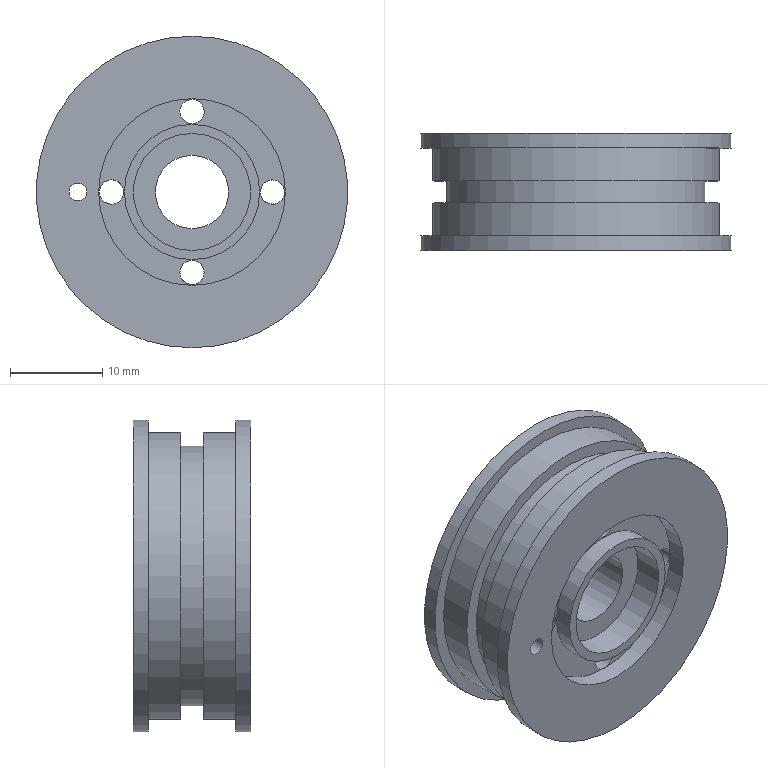Part | NX | features piston 2 | 1 solid | 23 faces | box 33.782 x 12.7 x 33.782 mm | volume 8306 mm3 | cylinder 14 | plane 9 | commonest cylinder face diameters 2.642 x4 31.115 x2 33.782 x2 1.93 x1 7.95 x1 12.7 x1
STEP:
#1=CARTESIAN_POINT('',(0.,0.,-7.333));
#2=VERTEX_POINT('',#1);
#3=CARTESIAN_POINT('',(0.,0.,0.));
#4=DIRECTION('',(0.,-1.,0.));
#5=DIRECTION('',(0.,0.,-1.));
#6=AXIS2_PLACEMENT_3D('',#3,#4,#5);
#7=CIRCLE('',#6,7.333);
#8=EDGE_CURVE('',#2,#2,#7,.F.);
#9=ORIENTED_EDGE('',*,*,#8,.F.);
#10=EDGE_LOOP('',(#9));
#11=FACE_BOUND('',#10,.T.);
#12=CARTESIAN_POINT('',(0.,0.,-6.35));
#13=VERTEX_POINT('',#12);
#14=CARTESIAN_POINT('',(0.,0.,0.));
#15=DIRECTION('',(0.,-1.,0.));
#16=DIRECTION('',(0.,0.,-1.));
#17=AXIS2_PLACEMENT_3D('',#14,#15,#16);
#18=CIRCLE('',#17,6.35);
#19=EDGE_CURVE('',#13,#13,#18,.T.);
#20=ORIENTED_EDGE('',*,*,#19,.F.);
#21=EDGE_LOOP('',(#20));
#22=FACE_BOUND('',#21,.T.);
#23=CARTESIAN_POINT('',(6.35,0.,0.));
#24=DIRECTION('',(0.,-1.,0.));
#25=DIRECTION('',(0.,0.,-1.));
#26=AXIS2_PLACEMENT_3D('',#23,#24,#25);
#27=PLANE('',#26);
#28=ADVANCED_FACE('',(#11,#22),#27,.T.);
#29=CARTESIAN_POINT('',(8.73,12.7,1.321));
#30=VERTEX_POINT('',#29);
#31=CARTESIAN_POINT('',(8.73,12.7,0.));
#32=DIRECTION('',(0.,1.,0.));
#33=DIRECTION('',(0.,0.,1.));
#34=AXIS2_PLACEMENT_3D('',#31,#32,#33);
#35=CIRCLE('',#34,1.321);
#36=EDGE_CURVE('',#30,#30,#35,.F.);
#37=ORIENTED_EDGE('',*,*,#36,.T.);
#38=EDGE_LOOP('',(#37));
#39=FACE_BOUND('',#38,.T.);
#40=CARTESIAN_POINT('',(-8.73,12.7,1.321));
#41=VERTEX_POINT('',#40);
#42=CARTESIAN_POINT('',(-8.73,12.7,0.));
#43=DIRECTION('',(0.,1.,0.));
#44=DIRECTION('',(0.,0.,1.));
#45=AXIS2_PLACEMENT_3D('',#42,#43,#44);
#46=CIRCLE('',#45,1.321);
#47=EDGE_CURVE('',#41,#41,#46,.F.);
#48=ORIENTED_EDGE('',*,*,#47,.T.);
#49=EDGE_LOOP('',(#48));
#50=FACE_BOUND('',#49,.T.);
#51=CARTESIAN_POINT('',(0.,12.7,-16.891));
#52=VERTEX_POINT('',#51);
#53=CARTESIAN_POINT('',(0.,12.7,0.));
#54=DIRECTION('',(0.,-1.,0.));
#55=DIRECTION('',(0.,0.,-1.));
#56=AXIS2_PLACEMENT_3D('',#53,#54,#55);
#57=CIRCLE('',#56,16.891);
#58=EDGE_CURVE('',#52,#52,#57,.T.);
#59=ORIENTED_EDGE('',*,*,#58,.F.);
#60=EDGE_LOOP('',(#59));
#61=FACE_BOUND('',#60,.T.);
#62=CARTESIAN_POINT('',(0.,12.7,-3.975));
#63=VERTEX_POINT('',#62);
#64=CARTESIAN_POINT('',(0.,12.7,0.));
#65=DIRECTION('',(0.,-1.,0.));
#66=DIRECTION('',(0.,0.,-1.));
#67=AXIS2_PLACEMENT_3D('',#64,#65,#66);
#68=CIRCLE('',#67,3.975);
#69=EDGE_CURVE('',#63,#63,#68,.T.);
#70=ORIENTED_EDGE('',*,*,#69,.T.);
#71=EDGE_LOOP('',(#70));
#72=FACE_BOUND('',#71,.T.);
#73=CARTESIAN_POINT('',(-12.383,12.7,0.9652));
#74=VERTEX_POINT('',#73);
#75=CARTESIAN_POINT('',(-12.383,12.7,0.));
#76=DIRECTION('',(0.,1.,0.));
#77=DIRECTION('',(0.,0.,1.));
#78=AXIS2_PLACEMENT_3D('',#75,#76,#77);
#79=CIRCLE('',#78,0.9652);
#80=EDGE_CURVE('',#74,#74,#79,.F.);
#81=ORIENTED_EDGE('',*,*,#80,.T.);
#82=EDGE_LOOP('',(#81));
#83=FACE_BOUND('',#82,.T.);
#84=CARTESIAN_POINT('',(0.,12.7,-7.409));
#85=VERTEX_POINT('',#84);
#86=CARTESIAN_POINT('',(0.,12.7,-8.73));
#87=DIRECTION('',(0.,1.,0.));
#88=DIRECTION('',(0.,0.,1.));
#89=AXIS2_PLACEMENT_3D('',#86,#87,#88);
#90=CIRCLE('',#89,1.321);
#91=EDGE_CURVE('',#85,#85,#90,.F.);
#92=ORIENTED_EDGE('',*,*,#91,.T.);
#93=EDGE_LOOP('',(#92));
#94=FACE_BOUND('',#93,.T.);
#95=CARTESIAN_POINT('',(0.,12.7,10.051));
#96=VERTEX_POINT('',#95);
#97=CARTESIAN_POINT('',(0.,12.7,8.73));
#98=DIRECTION('',(0.,1.,0.));
#99=DIRECTION('',(0.,0.,1.));
#100=AXIS2_PLACEMENT_3D('',#97,#98,#99);
#101=CIRCLE('',#100,1.321);
#102=EDGE_CURVE('',#96,#96,#101,.F.);
#103=ORIENTED_EDGE('',*,*,#102,.T.);
#104=EDGE_LOOP('',(#103));
#105=FACE_BOUND('',#104,.T.);
#106=CARTESIAN_POINT('',(16.891,12.7,0.));
#107=DIRECTION('',(0.,1.,0.));
#108=DIRECTION('',(0.,0.,1.));
#109=AXIS2_PLACEMENT_3D('',#106,#107,#108);
#110=PLANE('',#109);
#111=ADVANCED_FACE('',(#39,#50,#61,#72,#83,#94,#105),#110,.T.);
#112=CARTESIAN_POINT('',(0.,0.,-10.127));
#113=VERTEX_POINT('',#112);
#114=CARTESIAN_POINT('',(0.,0.,0.));
#115=DIRECTION('',(0.,-1.,0.));
#116=DIRECTION('',(0.,0.,-1.));
#117=AXIS2_PLACEMENT_3D('',#114,#115,#116);
#118=CIRCLE('',#117,10.127);
#119=EDGE_CURVE('',#113,#113,#118,.T.);
#120=ORIENTED_EDGE('',*,*,#119,.F.);
#121=EDGE_LOOP('',(#120));
#122=FACE_BOUND('',#121,.T.);
#123=CARTESIAN_POINT('',(0.,0.,-16.891));
#124=VERTEX_POINT('',#123);
#125=CARTESIAN_POINT('',(0.,0.,0.));
#126=DIRECTION('',(0.,-1.,0.));
#127=DIRECTION('',(0.,0.,-1.));
#128=AXIS2_PLACEMENT_3D('',#125,#126,#127);
#129=CIRCLE('',#128,16.891);
#130=EDGE_CURVE('',#124,#124,#129,.T.);
#131=ORIENTED_EDGE('',*,*,#130,.T.);
#132=EDGE_LOOP('',(#131));
#133=FACE_BOUND('',#132,.T.);
#134=CARTESIAN_POINT('',(-12.383,0.,-0.9652));
#135=VERTEX_POINT('',#134);
#136=CARTESIAN_POINT('',(-12.383,0.,0.));
#137=DIRECTION('',(0.,-1.,0.));
#138=DIRECTION('',(0.,0.,-1.));
#139=AXIS2_PLACEMENT_3D('',#136,#137,#138);
#140=CIRCLE('',#139,0.9652);
#141=EDGE_CURVE('',#135,#135,#140,.F.);
#142=ORIENTED_EDGE('',*,*,#141,.T.);
#143=EDGE_LOOP('',(#142));
#144=FACE_BOUND('',#143,.T.);
#145=CARTESIAN_POINT('',(6.35,0.,0.));
#146=DIRECTION('',(0.,-1.,0.));
#147=DIRECTION('',(0.,0.,-1.));
#148=AXIS2_PLACEMENT_3D('',#145,#146,#147);
#149=PLANE('',#148);
#150=ADVANCED_FACE('',(#122,#133,#144),#149,.T.);
#151=CARTESIAN_POINT('',(0.,3.175,-3.975));
#152=VERTEX_POINT('',#151);
#153=CARTESIAN_POINT('',(0.,3.175,0.));
#154=DIRECTION('',(0.,-1.,0.));
#155=DIRECTION('',(0.,0.,-1.));
#156=AXIS2_PLACEMENT_3D('',#153,#154,#155);
#157=CIRCLE('',#156,3.975);
#158=EDGE_CURVE('',#152,#152,#157,.T.);
#159=ORIENTED_EDGE('',*,*,#158,.T.);
#160=EDGE_LOOP('',(#159));
#161=FACE_BOUND('',#160,.T.);
#162=ORIENTED_EDGE('',*,*,#69,.F.);
#163=EDGE_LOOP('',(#162));
#164=FACE_BOUND('',#163,.T.);
#165=CARTESIAN_POINT('',(0.,0.,0.));
#166=DIRECTION('',(0.,-1.,0.));
#167=DIRECTION('',(0.,0.,-1.));
#168=AXIS2_PLACEMENT_3D('',#165,#166,#167);
#169=CYLINDRICAL_SURFACE('',#168,3.975);
#170=ADVANCED_FACE('',(#161,#164),#169,.F.);
#171=CARTESIAN_POINT('',(0.,3.175,-6.35));
#172=VERTEX_POINT('',#171);
#173=CARTESIAN_POINT('',(0.,3.175,0.));
#174=DIRECTION('',(0.,-1.,0.));
#175=DIRECTION('',(0.,0.,-1.));
#176=AXIS2_PLACEMENT_3D('',#173,#174,#175);
#177=CIRCLE('',#176,6.35);
#178=EDGE_CURVE('',#172,#172,#177,.T.);
#179=ORIENTED_EDGE('',*,*,#178,.T.);
#180=EDGE_LOOP('',(#179));
#181=FACE_BOUND('',#180,.T.);
#182=ORIENTED_EDGE('',*,*,#158,.F.);
#183=EDGE_LOOP('',(#182));
#184=FACE_BOUND('',#183,.T.);
#185=CARTESIAN_POINT('',(3.975,3.175,0.));
#186=DIRECTION('',(0.,-1.,0.));
#187=DIRECTION('',(0.,0.,-1.));
#188=AXIS2_PLACEMENT_3D('',#185,#186,#187);
#189=PLANE('',#188);
#190=ADVANCED_FACE('',(#181,#184),#189,.T.);
#191=ORIENTED_EDGE('',*,*,#19,.T.);
#192=EDGE_LOOP('',(#191));
#193=FACE_BOUND('',#192,.T.);
#194=ORIENTED_EDGE('',*,*,#178,.F.);
#195=EDGE_LOOP('',(#194));
#196=FACE_BOUND('',#195,.T.);
#197=CARTESIAN_POINT('',(0.,0.,0.));
#198=DIRECTION('',(0.,-1.,0.));
#199=DIRECTION('',(0.,0.,-1.));
#200=AXIS2_PLACEMENT_3D('',#197,#198,#199);
#201=CYLINDRICAL_SURFACE('',#200,6.35);
#202=ADVANCED_FACE('',(#193,#196),#201,.F.);
#203=CARTESIAN_POINT('',(0.,1.587,-16.891));
#204=VERTEX_POINT('',#203);
#205=CARTESIAN_POINT('',(0.,1.587,0.));
#206=DIRECTION('',(0.,-1.,0.));
#207=DIRECTION('',(0.,0.,-1.));
#208=AXIS2_PLACEMENT_3D('',#205,#206,#207);
#209=CIRCLE('',#208,16.891);
#210=EDGE_CURVE('',#204,#204,#209,.T.);
#211=ORIENTED_EDGE('',*,*,#210,.T.);
#212=EDGE_LOOP('',(#211));
#213=FACE_BOUND('',#212,.T.);
#214=ORIENTED_EDGE('',*,*,#130,.F.);
#215=EDGE_LOOP('',(#214));
#216=FACE_BOUND('',#215,.T.);
#217=CARTESIAN_POINT('',(0.,0.,0.));
#218=DIRECTION('',(0.,-1.,0.));
#219=DIRECTION('',(0.,0.,-1.));
#220=AXIS2_PLACEMENT_3D('',#217,#218,#219);
#221=CYLINDRICAL_SURFACE('',#220,16.891);
#222=ADVANCED_FACE('',(#213,#216),#221,.T.);
#223=CARTESIAN_POINT('',(0.,1.587,-15.557));
#224=VERTEX_POINT('',#223);
#225=CARTESIAN_POINT('',(0.,1.587,0.));
#226=DIRECTION('',(0.,-1.,0.));
#227=DIRECTION('',(0.,0.,-1.));
#228=AXIS2_PLACEMENT_3D('',#225,#226,#227);
#229=CIRCLE('',#228,15.557);
#230=EDGE_CURVE('',#224,#224,#229,.T.);
#231=ORIENTED_EDGE('',*,*,#230,.T.);
#232=EDGE_LOOP('',(#231));
#233=FACE_BOUND('',#232,.T.);
#234=ORIENTED_EDGE('',*,*,#210,.F.);
#235=EDGE_LOOP('',(#234));
#236=FACE_BOUND('',#235,.T.);
#237=CARTESIAN_POINT('',(16.891,1.587,0.));
#238=DIRECTION('',(0.,1.,0.));
#239=DIRECTION('',(0.,0.,1.));
#240=AXIS2_PLACEMENT_3D('',#237,#238,#239);
#241=PLANE('',#240);
#242=ADVANCED_FACE('',(#233,#236),#241,.T.);
#243=CARTESIAN_POINT('',(0.,5.156,-15.557));
#244=VERTEX_POINT('',#243);
#245=CARTESIAN_POINT('',(0.,5.156,0.));
#246=DIRECTION('',(0.,-1.,0.));
#247=DIRECTION('',(0.,0.,-1.));
#248=AXIS2_PLACEMENT_3D('',#245,#246,#247);
#249=CIRCLE('',#248,15.557);
#250=EDGE_CURVE('',#244,#244,#249,.T.);
#251=ORIENTED_EDGE('',*,*,#250,.T.);
#252=EDGE_LOOP('',(#251));
#253=FACE_BOUND('',#252,.T.);
#254=ORIENTED_EDGE('',*,*,#230,.F.);
#255=EDGE_LOOP('',(#254));
#256=FACE_BOUND('',#255,.T.);
#257=CARTESIAN_POINT('',(0.,0.,0.));
#258=DIRECTION('',(0.,-1.,0.));
#259=DIRECTION('',(0.,0.,-1.));
#260=AXIS2_PLACEMENT_3D('',#257,#258,#259);
#261=CYLINDRICAL_SURFACE('',#260,15.557);
#262=ADVANCED_FACE('',(#253,#256),#261,.T.);
#263=CARTESIAN_POINT('',(0.,5.156,-14.097));
#264=VERTEX_POINT('',#263);
#265=CARTESIAN_POINT('',(0.,5.156,0.));
#266=DIRECTION('',(0.,-1.,0.));
#267=DIRECTION('',(0.,0.,-1.));
#268=AXIS2_PLACEMENT_3D('',#265,#266,#267);
#269=CIRCLE('',#268,14.097);
#270=EDGE_CURVE('',#264,#264,#269,.T.);
#271=ORIENTED_EDGE('',*,*,#270,.T.);
#272=EDGE_LOOP('',(#271));
#273=FACE_BOUND('',#272,.T.);
#274=ORIENTED_EDGE('',*,*,#250,.F.);
#275=EDGE_LOOP('',(#274));
#276=FACE_BOUND('',#275,.T.);
#277=CARTESIAN_POINT('',(15.557,5.156,0.));
#278=DIRECTION('',(0.,1.,0.));
#279=DIRECTION('',(0.,0.,1.));
#280=AXIS2_PLACEMENT_3D('',#277,#278,#279);
#281=PLANE('',#280);
#282=ADVANCED_FACE('',(#273,#276),#281,.T.);
#283=CARTESIAN_POINT('',(0.,7.544,-14.097));
#284=VERTEX_POINT('',#283);
#285=CARTESIAN_POINT('',(0.,7.544,0.));
#286=DIRECTION('',(0.,-1.,0.));
#287=DIRECTION('',(0.,0.,-1.));
#288=AXIS2_PLACEMENT_3D('',#285,#286,#287);
#289=CIRCLE('',#288,14.097);
#290=EDGE_CURVE('',#284,#284,#289,.T.);
#291=ORIENTED_EDGE('',*,*,#290,.T.);
#292=EDGE_LOOP('',(#291));
#293=FACE_BOUND('',#292,.T.);
#294=ORIENTED_EDGE('',*,*,#270,.F.);
#295=EDGE_LOOP('',(#294));
#296=FACE_BOUND('',#295,.T.);
#297=CARTESIAN_POINT('',(0.,0.,0.));
#298=DIRECTION('',(0.,-1.,0.));
#299=DIRECTION('',(0.,0.,-1.));
#300=AXIS2_PLACEMENT_3D('',#297,#298,#299);
#301=CYLINDRICAL_SURFACE('',#300,14.097);
#302=ADVANCED_FACE('',(#293,#296),#301,.T.);
#303=CARTESIAN_POINT('',(0.,7.544,-15.557));
#304=VERTEX_POINT('',#303);
#305=CARTESIAN_POINT('',(0.,7.544,0.));
#306=DIRECTION('',(0.,-1.,0.));
#307=DIRECTION('',(0.,0.,-1.));
#308=AXIS2_PLACEMENT_3D('',#305,#306,#307);
#309=CIRCLE('',#308,15.557);
#310=EDGE_CURVE('',#304,#304,#309,.T.);
#311=ORIENTED_EDGE('',*,*,#310,.T.);
#312=EDGE_LOOP('',(#311));
#313=FACE_BOUND('',#312,.T.);
#314=ORIENTED_EDGE('',*,*,#290,.F.);
#315=EDGE_LOOP('',(#314));
#316=FACE_BOUND('',#315,.T.);
#317=CARTESIAN_POINT('',(14.097,7.544,0.));
#318=DIRECTION('',(0.,-1.,0.));
#319=DIRECTION('',(0.,0.,-1.));
#320=AXIS2_PLACEMENT_3D('',#317,#318,#319);
#321=PLANE('',#320);
#322=ADVANCED_FACE('',(#313,#316),#321,.T.);
#323=CARTESIAN_POINT('',(0.,11.113,-15.557));
#324=VERTEX_POINT('',#323);
#325=CARTESIAN_POINT('',(0.,11.113,0.));
#326=DIRECTION('',(0.,-1.,0.));
#327=DIRECTION('',(0.,0.,-1.));
#328=AXIS2_PLACEMENT_3D('',#325,#326,#327);
#329=CIRCLE('',#328,15.557);
#330=EDGE_CURVE('',#324,#324,#329,.T.);
#331=ORIENTED_EDGE('',*,*,#330,.T.);
#332=EDGE_LOOP('',(#331));
#333=FACE_BOUND('',#332,.T.);
#334=ORIENTED_EDGE('',*,*,#310,.F.);
#335=EDGE_LOOP('',(#334));
#336=FACE_BOUND('',#335,.T.);
#337=CARTESIAN_POINT('',(0.,0.,0.));
#338=DIRECTION('',(0.,-1.,0.));
#339=DIRECTION('',(0.,0.,-1.));
#340=AXIS2_PLACEMENT_3D('',#337,#338,#339);
#341=CYLINDRICAL_SURFACE('',#340,15.557);
#342=ADVANCED_FACE('',(#333,#336),#341,.T.);
#343=CARTESIAN_POINT('',(0.,11.113,-16.891));
#344=VERTEX_POINT('',#343);
#345=CARTESIAN_POINT('',(0.,11.113,0.));
#346=DIRECTION('',(0.,-1.,0.));
#347=DIRECTION('',(0.,0.,-1.));
#348=AXIS2_PLACEMENT_3D('',#345,#346,#347);
#349=CIRCLE('',#348,16.891);
#350=EDGE_CURVE('',#344,#344,#349,.T.);
#351=ORIENTED_EDGE('',*,*,#350,.T.);
#352=EDGE_LOOP('',(#351));
#353=FACE_BOUND('',#352,.T.);
#354=ORIENTED_EDGE('',*,*,#330,.F.);
#355=EDGE_LOOP('',(#354));
#356=FACE_BOUND('',#355,.T.);
#357=CARTESIAN_POINT('',(15.557,11.113,0.));
#358=DIRECTION('',(0.,-1.,0.));
#359=DIRECTION('',(0.,0.,-1.));
#360=AXIS2_PLACEMENT_3D('',#357,#358,#359);
#361=PLANE('',#360);
#362=ADVANCED_FACE('',(#353,#356),#361,.T.);
#363=ORIENTED_EDGE('',*,*,#58,.T.);
#364=EDGE_LOOP('',(#363));
#365=FACE_BOUND('',#364,.T.);
#366=ORIENTED_EDGE('',*,*,#350,.F.);
#367=EDGE_LOOP('',(#366));
#368=FACE_BOUND('',#367,.T.);
#369=CARTESIAN_POINT('',(0.,0.,0.));
#370=DIRECTION('',(0.,-1.,0.));
#371=DIRECTION('',(0.,0.,-1.));
#372=AXIS2_PLACEMENT_3D('',#369,#370,#371);
#373=CYLINDRICAL_SURFACE('',#372,16.891);
#374=ADVANCED_FACE('',(#365,#368),#373,.T.);
#375=ORIENTED_EDGE('',*,*,#80,.F.);
#376=EDGE_LOOP('',(#375));
#377=FACE_BOUND('',#376,.T.);
#378=ORIENTED_EDGE('',*,*,#141,.F.);
#379=EDGE_LOOP('',(#378));
#380=FACE_BOUND('',#379,.T.);
#381=CARTESIAN_POINT('',(-12.383,28.216,0.));
#382=DIRECTION('',(0.,1.,0.));
#383=DIRECTION('',(-1.,0.,0.));
#384=AXIS2_PLACEMENT_3D('',#381,#382,#383);
#385=CYLINDRICAL_SURFACE('',#384,0.9652);
#386=ADVANCED_FACE('',(#377,#380),#385,.F.);
#387=CARTESIAN_POINT('',(-10.051,2.032,0.));
#388=VERTEX_POINT('',#387);
#389=CARTESIAN_POINT('',(-8.73,2.032,0.));
#390=DIRECTION('',(0.,1.,0.));
#391=DIRECTION('',(-1.,0.,0.));
#392=AXIS2_PLACEMENT_3D('',#389,#390,#391);
#393=CIRCLE('',#392,1.321);
#394=EDGE_CURVE('',#388,#388,#393,.T.);
#395=ORIENTED_EDGE('',*,*,#394,.F.);
#396=EDGE_LOOP('',(#395));
#397=FACE_BOUND('',#396,.T.);
#398=ORIENTED_EDGE('',*,*,#47,.F.);
#399=EDGE_LOOP('',(#398));
#400=FACE_BOUND('',#399,.T.);
#401=CARTESIAN_POINT('',(-8.73,21.639,0.));
#402=DIRECTION('',(0.,1.,0.));
#403=DIRECTION('',(-1.,0.,0.));
#404=AXIS2_PLACEMENT_3D('',#401,#402,#403);
#405=CYLINDRICAL_SURFACE('',#404,1.321);
#406=ADVANCED_FACE('',(#397,#400),#405,.F.);
#407=CARTESIAN_POINT('',(-1.321,2.032,-8.73));
#408=VERTEX_POINT('',#407);
#409=CARTESIAN_POINT('',(0.,2.032,-8.73));
#410=DIRECTION('',(0.,1.,0.));
#411=DIRECTION('',(-1.,0.,0.));
#412=AXIS2_PLACEMENT_3D('',#409,#410,#411);
#413=CIRCLE('',#412,1.321);
#414=EDGE_CURVE('',#408,#408,#413,.T.);
#415=ORIENTED_EDGE('',*,*,#414,.F.);
#416=EDGE_LOOP('',(#415));
#417=FACE_BOUND('',#416,.T.);
#418=ORIENTED_EDGE('',*,*,#91,.F.);
#419=EDGE_LOOP('',(#418));
#420=FACE_BOUND('',#419,.T.);
#421=CARTESIAN_POINT('',(0.,21.639,-8.73));
#422=DIRECTION('',(0.,1.,0.));
#423=DIRECTION('',(0.,0.,-1.));
#424=AXIS2_PLACEMENT_3D('',#421,#422,#423);
#425=CYLINDRICAL_SURFACE('',#424,1.321);
#426=ADVANCED_FACE('',(#417,#420),#425,.F.);
#427=CARTESIAN_POINT('',(7.409,2.032,0.));
#428=VERTEX_POINT('',#427);
#429=CARTESIAN_POINT('',(8.73,2.032,0.));
#430=DIRECTION('',(0.,1.,0.));
#431=DIRECTION('',(-1.,0.,0.));
#432=AXIS2_PLACEMENT_3D('',#429,#430,#431);
#433=CIRCLE('',#432,1.321);
#434=EDGE_CURVE('',#428,#428,#433,.T.);
#435=ORIENTED_EDGE('',*,*,#434,.F.);
#436=EDGE_LOOP('',(#435));
#437=FACE_BOUND('',#436,.T.);
#438=ORIENTED_EDGE('',*,*,#36,.F.);
#439=EDGE_LOOP('',(#438));
#440=FACE_BOUND('',#439,.T.);
#441=CARTESIAN_POINT('',(8.73,21.639,0.));
#442=DIRECTION('',(0.,1.,0.));
#443=DIRECTION('',(1.,0.,0.));
#444=AXIS2_PLACEMENT_3D('',#441,#442,#443);
#445=CYLINDRICAL_SURFACE('',#444,1.321);
#446=ADVANCED_FACE('',(#437,#440),#445,.F.);
#447=CARTESIAN_POINT('',(-1.321,2.032,8.73));
#448=VERTEX_POINT('',#447);
#449=CARTESIAN_POINT('',(0.,2.032,8.73));
#450=DIRECTION('',(0.,1.,0.));
#451=DIRECTION('',(-1.,0.,0.));
#452=AXIS2_PLACEMENT_3D('',#449,#450,#451);
#453=CIRCLE('',#452,1.321);
#454=EDGE_CURVE('',#448,#448,#453,.T.);
#455=ORIENTED_EDGE('',*,*,#454,.F.);
#456=EDGE_LOOP('',(#455));
#457=FACE_BOUND('',#456,.T.);
#458=ORIENTED_EDGE('',*,*,#102,.F.);
#459=EDGE_LOOP('',(#458));
#460=FACE_BOUND('',#459,.T.);
#461=CARTESIAN_POINT('',(0.,21.639,8.73));
#462=DIRECTION('',(0.,1.,0.));
#463=DIRECTION('',(0.,0.,1.));
#464=AXIS2_PLACEMENT_3D('',#461,#462,#463);
#465=CYLINDRICAL_SURFACE('',#464,1.321);
#466=ADVANCED_FACE('',(#457,#460),#465,.F.);
#467=ORIENTED_EDGE('',*,*,#8,.T.);
#468=EDGE_LOOP('',(#467));
#469=FACE_BOUND('',#468,.T.);
#470=CARTESIAN_POINT('',(7.333,2.032,0.));
#471=VERTEX_POINT('',#470);
#472=CARTESIAN_POINT('',(0.,2.032,0.));
#473=DIRECTION('',(0.,-1.,0.));
#474=DIRECTION('',(1.,0.,0.));
#475=AXIS2_PLACEMENT_3D('',#472,#473,#474);
#476=CIRCLE('',#475,7.333);
#477=EDGE_CURVE('',#471,#471,#476,.T.);
#478=ORIENTED_EDGE('',*,*,#477,.T.);
#479=EDGE_LOOP('',(#478));
#480=FACE_BOUND('',#479,.T.);
#481=CARTESIAN_POINT('',(0.,4.463,0.));
#482=DIRECTION('',(0.,-1.,0.));
#483=DIRECTION('',(1.,0.,0.));
#484=AXIS2_PLACEMENT_3D('',#481,#482,#483);
#485=CYLINDRICAL_SURFACE('',#484,7.333);
#486=ADVANCED_FACE('',(#469,#480),#485,.T.);
#487=ORIENTED_EDGE('',*,*,#119,.T.);
#488=EDGE_LOOP('',(#487));
#489=FACE_BOUND('',#488,.T.);
#490=CARTESIAN_POINT('',(10.127,2.032,0.));
#491=VERTEX_POINT('',#490);
#492=CARTESIAN_POINT('',(0.,2.032,0.));
#493=DIRECTION('',(0.,-1.,0.));
#494=DIRECTION('',(1.,0.,0.));
#495=AXIS2_PLACEMENT_3D('',#492,#493,#494);
#496=CIRCLE('',#495,10.127);
#497=EDGE_CURVE('',#491,#491,#496,.T.);
#498=ORIENTED_EDGE('',*,*,#497,.F.);
#499=EDGE_LOOP('',(#498));
#500=FACE_BOUND('',#499,.T.);
#501=CARTESIAN_POINT('',(0.,4.463,0.));
#502=DIRECTION('',(0.,-1.,0.));
#503=DIRECTION('',(1.,0.,0.));
#504=AXIS2_PLACEMENT_3D('',#501,#502,#503);
#505=CYLINDRICAL_SURFACE('',#504,10.127);
#506=ADVANCED_FACE('',(#489,#500),#505,.F.);
#507=ORIENTED_EDGE('',*,*,#394,.T.);
#508=EDGE_LOOP('',(#507));
#509=FACE_BOUND('',#508,.T.);
#510=ORIENTED_EDGE('',*,*,#414,.T.);
#511=EDGE_LOOP('',(#510));
#512=FACE_BOUND('',#511,.T.);
#513=ORIENTED_EDGE('',*,*,#434,.T.);
#514=EDGE_LOOP('',(#513));
#515=FACE_BOUND('',#514,.T.);
#516=ORIENTED_EDGE('',*,*,#454,.T.);
#517=EDGE_LOOP('',(#516));
#518=FACE_BOUND('',#517,.T.);
#519=ORIENTED_EDGE('',*,*,#477,.F.);
#520=EDGE_LOOP('',(#519));
#521=FACE_BOUND('',#520,.T.);
#522=ORIENTED_EDGE('',*,*,#497,.T.);
#523=EDGE_LOOP('',(#522));
#524=FACE_BOUND('',#523,.T.);
#525=CARTESIAN_POINT('',(7.333,2.032,0.));
#526=DIRECTION('',(0.,1.,0.));
#527=DIRECTION('',(-1.,0.,0.));
#528=AXIS2_PLACEMENT_3D('',#525,#526,#527);
#529=PLANE('',#528);
#530=ADVANCED_FACE('',(#509,#512,#515,#518,#521,#524),#529,.F.);
#531=CLOSED_SHELL('',(#28,#111,#150,#170,#190,#202,#222,#242,#262,#282,#302,#322,#342,#362,#374,#386,#406,#426,#446,#466,#486,#506,#530));
#532=MANIFOLD_SOLID_BREP('',#531);
#533=(LENGTH_UNIT()NAMED_UNIT(*)SI_UNIT(.MILLI.,.METRE.));
#534=UNCERTAINTY_MEASURE_WITH_UNIT(LENGTH_MEASURE(0.00001),#533,'','');
#535=(NAMED_UNIT(*)PLANE_ANGLE_UNIT()SI_UNIT($,.RADIAN.));
#536=(NAMED_UNIT(*)SI_UNIT($,.STERADIAN.)SOLID_ANGLE_UNIT());
#537=(GEOMETRIC_REPRESENTATION_CONTEXT(3)GLOBAL_UNCERTAINTY_ASSIGNED_CONTEXT((#534))GLOBAL_UNIT_ASSIGNED_CONTEXT((#533,#535,#536))REPRESENTATION_CONTEXT('',''));
#538=ADVANCED_BREP_SHAPE_REPRESENTATION('',(#532),#537);